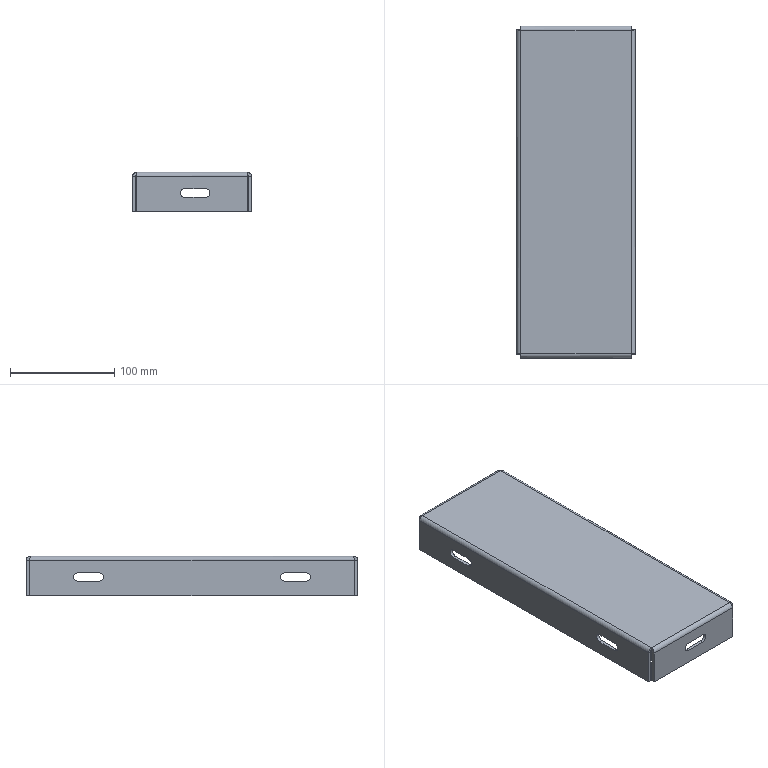Part | NX | features BREP 1 | 1 solid | 62 faces | box 114.1 x 319 x 38 mm | volume 190079 mm3 | plane 34 | cylinder 20 | spline 8 | commonest cylinder face diameters 8.5 x12 2 x4 8 x4